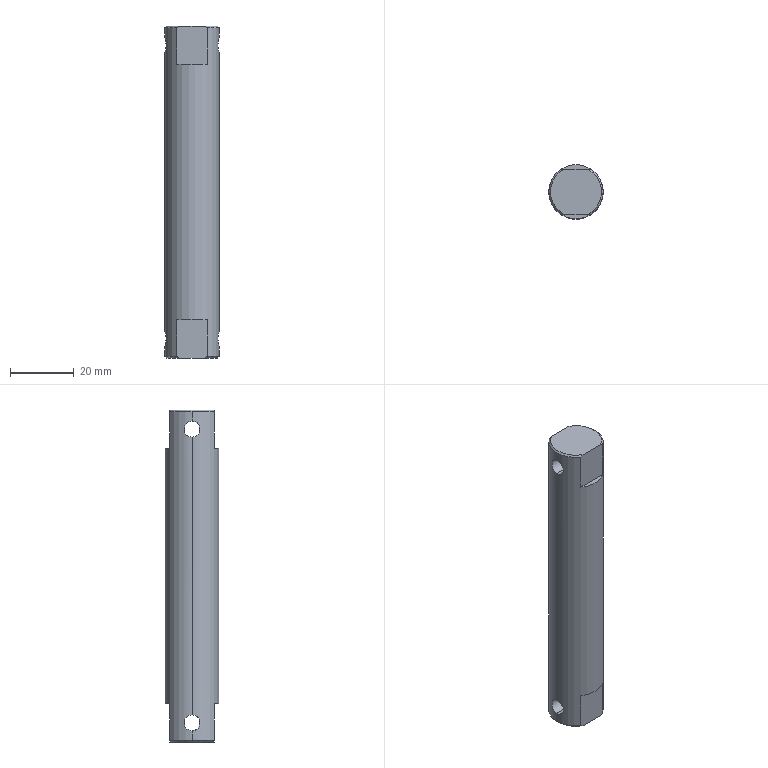Part | SolidWorks | features Chamfer 1, Extrusion 1, HoleWzd 1, ICE 1, MirrorPattern 1 | 1 solid | 22 faces | box 17 x 17 x 104 mm | volume 22466 mm3 | plane 10 | cylinder 6 | cone 6 | commonest cylinder face diameters 5 x4 17 x2
STEP:
#1=CARTESIAN_POINT('',(-8.5,0.,48.5));
#2=VERTEX_POINT('',#1);
#3=CARTESIAN_POINT('',(-8.5,0.,43.5));
#4=VERTEX_POINT('',#3);
#5=CARTESIAN_POINT('',(-8.5,0.,48.5));
#6=CARTESIAN_POINT('',(-8.5,-0.3274,48.5));
#7=CARTESIAN_POINT('',(-8.48,-0.658,48.434));
#8=CARTESIAN_POINT('',(-8.429,-1.11,48.246));
#9=CARTESIAN_POINT('',(-8.408,-1.256,48.168));
#10=CARTESIAN_POINT('',(-8.363,-1.527,47.986));
#11=CARTESIAN_POINT('',(-8.339,-1.652,47.883));
#12=CARTESIAN_POINT('',(-8.29,-1.883,47.653));
#13=CARTESIAN_POINT('',(-8.265,-1.987,47.525));
#14=CARTESIAN_POINT('',(-8.219,-2.168,47.256));
#15=CARTESIAN_POINT('',(-8.198,-2.245,47.113));
#16=CARTESIAN_POINT('',(-8.163,-2.372,46.808));
#17=CARTESIAN_POINT('',(-8.149,-2.419,46.651));
#18=CARTESIAN_POINT('',(-8.129,-2.483,46.331));
#19=CARTESIAN_POINT('',(-8.124,-2.5,46.165));
#20=CARTESIAN_POINT('',(-8.124,-2.5,45.835));
#21=CARTESIAN_POINT('',(-8.129,-2.484,45.673));
#22=CARTESIAN_POINT('',(-8.148,-2.42,45.351));
#23=CARTESIAN_POINT('',(-8.163,-2.371,45.191));
#24=CARTESIAN_POINT('',(-8.216,-2.183,44.739));
#25=CARTESIAN_POINT('',(-8.265,-1.998,44.462));
#26=CARTESIAN_POINT('',(-8.338,-1.654,44.118));
#27=CARTESIAN_POINT('',(-8.363,-1.527,44.013));
#28=CARTESIAN_POINT('',(-8.408,-1.255,43.832));
#29=CARTESIAN_POINT('',(-8.428,-1.112,43.755));
#30=CARTESIAN_POINT('',(-8.463,-0.8109,43.63));
#31=CARTESIAN_POINT('',(-8.477,-0.6512,43.581));
#32=CARTESIAN_POINT('',(-8.495,-0.3296,43.516));
#33=CARTESIAN_POINT('',(-8.5,-0.1661,43.5));
#34=CARTESIAN_POINT('',(-8.5,0.,43.5));
#35=B_SPLINE_CURVE_WITH_KNOTS('',3,(#5,#6,#7,#8,#9,#10,#11,#12,#13,#14,#15,#16,#17,#18,#19,#20,#21,#22,#23,#24,#25,#26,#27,#28,#29,#30,#31,#32,#33,#34),.UNSPECIFIED.,.F.,.F.,(4,2,2,2,2,2,2,2,2,2,2,2,2,2,4),(0.00786,0.008842,0.009333,0.009824,0.01032,0.01081,0.0113,0.01179,0.01228,0.01277,0.01375,0.01424,0.01474,0.01523,0.01572),.UNSPECIFIED.);
#36=EDGE_CURVE('',#2,#4,#35,.T.);
#37=ORIENTED_EDGE('',*,*,#36,.F.);
#38=CARTESIAN_POINT('',(8.5,0.,48.5));
#39=VERTEX_POINT('',#38);
#40=CARTESIAN_POINT('',(8.5,0.,48.5));
#41=DIRECTION('',(1.,0.,0.));
#42=VECTOR('',#41,1000.);
#43=LINE('',#40,#42);
#44=EDGE_CURVE('',#2,#39,#43,.T.);
#45=ORIENTED_EDGE('',*,*,#44,.T.);
#46=CARTESIAN_POINT('',(8.5,0.,43.5));
#47=VERTEX_POINT('',#46);
#48=CARTESIAN_POINT('',(8.5,0.,43.5));
#49=CARTESIAN_POINT('',(8.5,-0.1662,43.5));
#50=CARTESIAN_POINT('',(8.495,-0.3294,43.516));
#51=CARTESIAN_POINT('',(8.477,-0.6502,43.58));
#52=CARTESIAN_POINT('',(8.463,-0.8095,43.629));
#53=CARTESIAN_POINT('',(8.428,-1.112,43.755));
#54=CARTESIAN_POINT('',(8.408,-1.255,43.832));
#55=CARTESIAN_POINT('',(8.363,-1.526,44.013));
#56=CARTESIAN_POINT('',(8.338,-1.654,44.118));
#57=CARTESIAN_POINT('',(8.265,-1.998,44.462));
#58=CARTESIAN_POINT('',(8.216,-2.183,44.74));
#59=CARTESIAN_POINT('',(8.163,-2.371,45.19));
#60=CARTESIAN_POINT('',(8.149,-2.419,45.349));
#61=CARTESIAN_POINT('',(8.129,-2.484,45.672));
#62=CARTESIAN_POINT('',(8.124,-2.5,45.835));
#63=CARTESIAN_POINT('',(8.124,-2.5,46.163));
#64=CARTESIAN_POINT('',(8.129,-2.484,46.33));
#65=CARTESIAN_POINT('',(8.149,-2.419,46.651));
#66=CARTESIAN_POINT('',(8.163,-2.372,46.807));
#67=CARTESIAN_POINT('',(8.216,-2.182,47.263));
#68=CARTESIAN_POINT('',(8.265,-1.998,47.538));
#69=CARTESIAN_POINT('',(8.339,-1.652,47.884));
#70=CARTESIAN_POINT('',(8.363,-1.526,47.987));
#71=CARTESIAN_POINT('',(8.408,-1.256,48.168));
#72=CARTESIAN_POINT('',(8.429,-1.11,48.246));
#73=CARTESIAN_POINT('',(8.463,-0.8084,48.371));
#74=CARTESIAN_POINT('',(8.476,-0.6525,48.419));
#75=CARTESIAN_POINT('',(8.495,-0.3297,48.484));
#76=CARTESIAN_POINT('',(8.5,-0.1637,48.5));
#77=CARTESIAN_POINT('',(8.5,0.,48.5));
#78=B_SPLINE_CURVE_WITH_KNOTS('',3,(#48,#49,#50,#51,#52,#53,#54,#55,#56,#57,#58,#59,#60,#61,#62,#63,#64,#65,#66,#67,#68,#69,#70,#71,#72,#73,#74,#75,#76,#77),.UNSPECIFIED.,.F.,.F.,(4,2,2,2,2,2,2,2,2,2,2,2,2,2,4),(0.,0.0004912,0.0009825,0.001474,0.001965,0.002947,0.003439,0.00393,0.004421,0.004912,0.005895,0.006386,0.006877,0.007369,0.00786),.UNSPECIFIED.);
#79=EDGE_CURVE('',#47,#39,#78,.T.);
#80=ORIENTED_EDGE('',*,*,#79,.F.);
#81=CARTESIAN_POINT('',(8.5,0.,43.5));
#82=DIRECTION('',(1.,0.,0.));
#83=VECTOR('',#82,1000.);
#84=LINE('',#81,#83);
#85=EDGE_CURVE('',#4,#47,#84,.T.);
#86=ORIENTED_EDGE('',*,*,#85,.F.);
#87=EDGE_LOOP('',(#37,#45,#80,#86));
#88=FACE_OUTER_BOUND('',#87,.T.);
#89=CARTESIAN_POINT('',(8.5,0.,46.));
#90=DIRECTION('',(1.,0.,0.));
#91=DIRECTION('',(0.,0.,-1.));
#92=AXIS2_PLACEMENT_3D('',#89,#90,#91);
#93=CYLINDRICAL_SURFACE('',#92,2.5);
#94=ADVANCED_FACE('',(#88),#93,.F.);
#95=CARTESIAN_POINT('',(-8.5,0.,-43.5));
#96=VERTEX_POINT('',#95);
#97=CARTESIAN_POINT('',(-8.5,0.,-48.5));
#98=VERTEX_POINT('',#97);
#99=CARTESIAN_POINT('',(-8.5,0.,-43.5));
#100=CARTESIAN_POINT('',(-8.5,-0.3274,-43.5));
#101=CARTESIAN_POINT('',(-8.48,-0.658,-43.566));
#102=CARTESIAN_POINT('',(-8.429,-1.11,-43.754));
#103=CARTESIAN_POINT('',(-8.408,-1.256,-43.832));
#104=CARTESIAN_POINT('',(-8.363,-1.527,-44.014));
#105=CARTESIAN_POINT('',(-8.339,-1.652,-44.117));
#106=CARTESIAN_POINT('',(-8.29,-1.883,-44.347));
#107=CARTESIAN_POINT('',(-8.265,-1.987,-44.475));
#108=CARTESIAN_POINT('',(-8.219,-2.168,-44.744));
#109=CARTESIAN_POINT('',(-8.198,-2.245,-44.887));
#110=CARTESIAN_POINT('',(-8.163,-2.372,-45.192));
#111=CARTESIAN_POINT('',(-8.149,-2.419,-45.349));
#112=CARTESIAN_POINT('',(-8.129,-2.483,-45.669));
#113=CARTESIAN_POINT('',(-8.124,-2.5,-45.835));
#114=CARTESIAN_POINT('',(-8.124,-2.5,-46.165));
#115=CARTESIAN_POINT('',(-8.129,-2.484,-46.327));
#116=CARTESIAN_POINT('',(-8.148,-2.42,-46.649));
#117=CARTESIAN_POINT('',(-8.163,-2.371,-46.809));
#118=CARTESIAN_POINT('',(-8.216,-2.183,-47.261));
#119=CARTESIAN_POINT('',(-8.265,-1.998,-47.538));
#120=CARTESIAN_POINT('',(-8.338,-1.654,-47.882));
#121=CARTESIAN_POINT('',(-8.363,-1.527,-47.987));
#122=CARTESIAN_POINT('',(-8.408,-1.255,-48.168));
#123=CARTESIAN_POINT('',(-8.428,-1.112,-48.245));
#124=CARTESIAN_POINT('',(-8.463,-0.8109,-48.37));
#125=CARTESIAN_POINT('',(-8.477,-0.6512,-48.419));
#126=CARTESIAN_POINT('',(-8.495,-0.3296,-48.484));
#127=CARTESIAN_POINT('',(-8.5,-0.1661,-48.5));
#128=CARTESIAN_POINT('',(-8.5,0.,-48.5));
#129=B_SPLINE_CURVE_WITH_KNOTS('',3,(#99,#100,#101,#102,#103,#104,#105,#106,#107,#108,#109,#110,#111,#112,#113,#114,#115,#116,#117,#118,#119,#120,#121,#122,#123,#124,#125,#126,#127,#128),.UNSPECIFIED.,.F.,.F.,(4,2,2,2,2,2,2,2,2,2,2,2,2,2,4),(0.00786,0.008842,0.009333,0.009824,0.01032,0.01081,0.0113,0.01179,0.01228,0.01277,0.01375,0.01424,0.01474,0.01523,0.01572),.UNSPECIFIED.);
#130=EDGE_CURVE('',#96,#98,#129,.T.);
#131=ORIENTED_EDGE('',*,*,#130,.F.);
#132=CARTESIAN_POINT('',(8.5,0.,-43.5));
#133=VERTEX_POINT('',#132);
#134=CARTESIAN_POINT('',(8.5,0.,-43.5));
#135=DIRECTION('',(1.,0.,0.));
#136=VECTOR('',#135,1000.);
#137=LINE('',#134,#136);
#138=EDGE_CURVE('',#96,#133,#137,.T.);
#139=ORIENTED_EDGE('',*,*,#138,.T.);
#140=CARTESIAN_POINT('',(8.5,0.,-48.5));
#141=VERTEX_POINT('',#140);
#142=CARTESIAN_POINT('',(8.5,0.,-48.5));
#143=CARTESIAN_POINT('',(8.5,-0.1662,-48.5));
#144=CARTESIAN_POINT('',(8.495,-0.3294,-48.484));
#145=CARTESIAN_POINT('',(8.477,-0.6502,-48.42));
#146=CARTESIAN_POINT('',(8.463,-0.8095,-48.371));
#147=CARTESIAN_POINT('',(8.428,-1.112,-48.245));
#148=CARTESIAN_POINT('',(8.408,-1.255,-48.168));
#149=CARTESIAN_POINT('',(8.363,-1.526,-47.987));
#150=CARTESIAN_POINT('',(8.338,-1.654,-47.882));
#151=CARTESIAN_POINT('',(8.265,-1.998,-47.538));
#152=CARTESIAN_POINT('',(8.216,-2.183,-47.26));
#153=CARTESIAN_POINT('',(8.163,-2.371,-46.81));
#154=CARTESIAN_POINT('',(8.149,-2.419,-46.651));
#155=CARTESIAN_POINT('',(8.129,-2.484,-46.328));
#156=CARTESIAN_POINT('',(8.124,-2.5,-46.165));
#157=CARTESIAN_POINT('',(8.124,-2.5,-45.837));
#158=CARTESIAN_POINT('',(8.129,-2.484,-45.67));
#159=CARTESIAN_POINT('',(8.149,-2.419,-45.349));
#160=CARTESIAN_POINT('',(8.163,-2.372,-45.193));
#161=CARTESIAN_POINT('',(8.216,-2.182,-44.737));
#162=CARTESIAN_POINT('',(8.265,-1.998,-44.462));
#163=CARTESIAN_POINT('',(8.339,-1.652,-44.116));
#164=CARTESIAN_POINT('',(8.363,-1.526,-44.013));
#165=CARTESIAN_POINT('',(8.408,-1.256,-43.832));
#166=CARTESIAN_POINT('',(8.429,-1.11,-43.754));
#167=CARTESIAN_POINT('',(8.463,-0.8084,-43.629));
#168=CARTESIAN_POINT('',(8.476,-0.6525,-43.581));
#169=CARTESIAN_POINT('',(8.495,-0.3297,-43.516));
#170=CARTESIAN_POINT('',(8.5,-0.1637,-43.5));
#171=CARTESIAN_POINT('',(8.5,0.,-43.5));
#172=B_SPLINE_CURVE_WITH_KNOTS('',3,(#142,#143,#144,#145,#146,#147,#148,#149,#150,#151,#152,#153,#154,#155,#156,#157,#158,#159,#160,#161,#162,#163,#164,#165,#166,#167,#168,#169,#170,#171),.UNSPECIFIED.,.F.,.F.,(4,2,2,2,2,2,2,2,2,2,2,2,2,2,4),(0.,0.0004912,0.0009825,0.001474,0.001965,0.002947,0.003439,0.00393,0.004421,0.004912,0.005895,0.006386,0.006877,0.007369,0.00786),.UNSPECIFIED.);
#173=EDGE_CURVE('',#141,#133,#172,.T.);
#174=ORIENTED_EDGE('',*,*,#173,.F.);
#175=CARTESIAN_POINT('',(8.5,0.,-48.5));
#176=DIRECTION('',(1.,0.,0.));
#177=VECTOR('',#176,1000.);
#178=LINE('',#175,#177);
#179=EDGE_CURVE('',#98,#141,#178,.T.);
#180=ORIENTED_EDGE('',*,*,#179,.F.);
#181=EDGE_LOOP('',(#131,#139,#174,#180));
#182=FACE_OUTER_BOUND('',#181,.T.);
#183=CARTESIAN_POINT('',(8.5,0.,-46.));
#184=DIRECTION('',(1.,0.,0.));
#185=DIRECTION('',(0.,0.,-1.));
#186=AXIS2_PLACEMENT_3D('',#183,#184,#185);
#187=CYLINDRICAL_SURFACE('',#186,2.5);
#188=ADVANCED_FACE('',(#182),#187,.F.);
#189=CARTESIAN_POINT('',(-8.,0.,52.));
#190=VERTEX_POINT('',#189);
#191=CARTESIAN_POINT('',(-3.873,-7.,52.));
#192=VERTEX_POINT('',#191);
#193=CARTESIAN_POINT('',(0.,0.,52.));
#194=DIRECTION('',(0.,0.,1.));
#195=DIRECTION('',(1.,0.,0.));
#196=AXIS2_PLACEMENT_3D('',#193,#194,#195);
#197=CIRCLE('',#196,8.);
#198=EDGE_CURVE('',#190,#192,#197,.T.);
#199=ORIENTED_EDGE('',*,*,#198,.F.);
#200=CARTESIAN_POINT('',(-8.5,0.,51.5));
#201=VERTEX_POINT('',#200);
#202=CARTESIAN_POINT('',(-8.,0.,52.));
#203=DIRECTION('',(-0.7071,0.,-0.7071));
#204=VECTOR('',#203,1000.);
#205=LINE('',#202,#204);
#206=EDGE_CURVE('',#190,#201,#205,.T.);
#207=ORIENTED_EDGE('',*,*,#206,.T.);
#208=CARTESIAN_POINT('',(-4.822,-7.,51.5));
#209=VERTEX_POINT('',#208);
#210=CARTESIAN_POINT('',(0.,0.,51.5));
#211=DIRECTION('',(0.,0.,-1.));
#212=DIRECTION('',(1.,0.,0.));
#213=AXIS2_PLACEMENT_3D('',#210,#211,#212);
#214=CIRCLE('',#213,8.5);
#215=EDGE_CURVE('',#209,#201,#214,.T.);
#216=ORIENTED_EDGE('',*,*,#215,.F.);
#217=CARTESIAN_POINT('',(-3.873,-7.,52.));
#218=CARTESIAN_POINT('',(-4.195,-7.,51.844));
#219=CARTESIAN_POINT('',(-4.511,-7.,51.676));
#220=CARTESIAN_POINT('',(-4.822,-7.,51.5));
#221=B_SPLINE_CURVE_WITH_KNOTS('',3,(#217,#218,#219,#220),.UNSPECIFIED.,.F.,.F.,(4,4),(0.,0.001073),.UNSPECIFIED.);
#222=EDGE_CURVE('',#192,#209,#221,.T.);
#223=ORIENTED_EDGE('',*,*,#222,.F.);
#224=EDGE_LOOP('',(#199,#207,#216,#223));
#225=FACE_OUTER_BOUND('',#224,.T.);
#226=CARTESIAN_POINT('',(0.,0.,52.));
#227=DIRECTION('',(0.,0.,-1.));
#228=DIRECTION('',(-1.,0.,0.));
#229=AXIS2_PLACEMENT_3D('',#226,#227,#228);
#230=CONICAL_SURFACE('',#229,8.,0.7854);
#231=ADVANCED_FACE('',(#225),#230,.T.);
#232=CARTESIAN_POINT('',(8.,0.,-52.));
#233=VERTEX_POINT('',#232);
#234=CARTESIAN_POINT('',(3.873,-7.,-52.));
#235=VERTEX_POINT('',#234);
#236=CARTESIAN_POINT('',(0.,0.,-52.));
#237=DIRECTION('',(0.,0.,-1.));
#238=DIRECTION('',(1.,0.,0.));
#239=AXIS2_PLACEMENT_3D('',#236,#237,#238);
#240=CIRCLE('',#239,8.);
#241=EDGE_CURVE('',#233,#235,#240,.T.);
#242=ORIENTED_EDGE('',*,*,#241,.F.);
#243=CARTESIAN_POINT('',(8.5,0.,-51.5));
#244=VERTEX_POINT('',#243);
#245=CARTESIAN_POINT('',(8.5,0.,-51.5));
#246=DIRECTION('',(0.7071,0.,0.7071));
#247=VECTOR('',#246,1000.);
#248=LINE('',#245,#247);
#249=EDGE_CURVE('',#233,#244,#248,.T.);
#250=ORIENTED_EDGE('',*,*,#249,.T.);
#251=CARTESIAN_POINT('',(4.822,-7.,-51.5));
#252=VERTEX_POINT('',#251);
#253=CARTESIAN_POINT('',(0.,0.,-51.5));
#254=DIRECTION('',(0.,0.,1.));
#255=DIRECTION('',(1.,0.,0.));
#256=AXIS2_PLACEMENT_3D('',#253,#254,#255);
#257=CIRCLE('',#256,8.5);
#258=EDGE_CURVE('',#252,#244,#257,.T.);
#259=ORIENTED_EDGE('',*,*,#258,.F.);
#260=CARTESIAN_POINT('',(3.873,-7.,-52.));
#261=CARTESIAN_POINT('',(4.195,-7.,-51.844));
#262=CARTESIAN_POINT('',(4.511,-7.,-51.676));
#263=CARTESIAN_POINT('',(4.822,-7.,-51.5));
#264=B_SPLINE_CURVE_WITH_KNOTS('',3,(#260,#261,#262,#263),.UNSPECIFIED.,.F.,.F.,(4,4),(0.,0.001073),.UNSPECIFIED.);
#265=EDGE_CURVE('',#235,#252,#264,.T.);
#266=ORIENTED_EDGE('',*,*,#265,.F.);
#267=EDGE_LOOP('',(#242,#250,#259,#266));
#268=FACE_OUTER_BOUND('',#267,.T.);
#269=CARTESIAN_POINT('',(0.,0.,-51.5));
#270=DIRECTION('',(0.,0.,1.));
#271=DIRECTION('',(1.,0.,0.));
#272=AXIS2_PLACEMENT_3D('',#269,#270,#271);
#273=CONICAL_SURFACE('',#272,8.5,0.7854);
#274=ADVANCED_FACE('',(#268),#273,.T.);
#275=CARTESIAN_POINT('',(4.822,7.,51.5));
#276=VERTEX_POINT('',#275);
#277=CARTESIAN_POINT('',(8.5,0.,51.5));
#278=VERTEX_POINT('',#277);
#279=CARTESIAN_POINT('',(0.,0.,51.5));
#280=DIRECTION('',(0.,0.,-1.));
#281=DIRECTION('',(1.,0.,0.));
#282=AXIS2_PLACEMENT_3D('',#279,#280,#281);
#283=CIRCLE('',#282,8.5);
#284=EDGE_CURVE('',#276,#278,#283,.T.);
#285=ORIENTED_EDGE('',*,*,#284,.T.);
#286=CARTESIAN_POINT('',(8.5,0.,52.));
#287=DIRECTION('',(0.,0.,-1.));
#288=VECTOR('',#287,1000.);
#289=LINE('',#286,#288);
#290=EDGE_CURVE('',#278,#39,#289,.T.);
#291=ORIENTED_EDGE('',*,*,#290,.T.);
#292=CARTESIAN_POINT('',(8.5,0.,48.5));
#293=CARTESIAN_POINT('',(8.5,0.3274,48.5));
#294=CARTESIAN_POINT('',(8.48,0.658,48.434));
#295=CARTESIAN_POINT('',(8.429,1.11,48.246));
#296=CARTESIAN_POINT('',(8.408,1.256,48.168));
#297=CARTESIAN_POINT('',(8.363,1.527,47.986));
#298=CARTESIAN_POINT('',(8.339,1.652,47.883));
#299=CARTESIAN_POINT('',(8.29,1.883,47.653));
#300=CARTESIAN_POINT('',(8.265,1.987,47.525));
#301=CARTESIAN_POINT('',(8.219,2.168,47.256));
#302=CARTESIAN_POINT('',(8.198,2.245,47.113));
#303=CARTESIAN_POINT('',(8.163,2.372,46.808));
#304=CARTESIAN_POINT('',(8.149,2.419,46.651));
#305=CARTESIAN_POINT('',(8.129,2.483,46.331));
#306=CARTESIAN_POINT('',(8.124,2.5,46.165));
#307=CARTESIAN_POINT('',(8.124,2.5,45.835));
#308=CARTESIAN_POINT('',(8.129,2.484,45.673));
#309=CARTESIAN_POINT('',(8.148,2.42,45.351));
#310=CARTESIAN_POINT('',(8.163,2.371,45.191));
#311=CARTESIAN_POINT('',(8.216,2.183,44.739));
#312=CARTESIAN_POINT('',(8.265,1.998,44.462));
#313=CARTESIAN_POINT('',(8.338,1.654,44.118));
#314=CARTESIAN_POINT('',(8.363,1.527,44.013));
#315=CARTESIAN_POINT('',(8.408,1.255,43.832));
#316=CARTESIAN_POINT('',(8.428,1.112,43.755));
#317=CARTESIAN_POINT('',(8.463,0.8109,43.63));
#318=CARTESIAN_POINT('',(8.477,0.6512,43.581));
#319=CARTESIAN_POINT('',(8.495,0.3296,43.516));
#320=CARTESIAN_POINT('',(8.5,0.1661,43.5));
#321=CARTESIAN_POINT('',(8.5,0.,43.5));
#322=B_SPLINE_CURVE_WITH_KNOTS('',3,(#292,#293,#294,#295,#296,#297,#298,#299,#300,#301,#302,#303,#304,#305,#306,#307,#308,#309,#310,#311,#312,#313,#314,#315,#316,#317,#318,#319,#320,#321),.UNSPECIFIED.,.F.,.F.,(4,2,2,2,2,2,2,2,2,2,2,2,2,2,4),(0.00786,0.008842,0.009333,0.009824,0.01032,0.01081,0.0113,0.01179,0.01228,0.01277,0.01375,0.01424,0.01474,0.01523,0.01572),.UNSPECIFIED.);
#323=EDGE_CURVE('',#39,#47,#322,.T.);
#324=ORIENTED_EDGE('',*,*,#323,.T.);
#325=CARTESIAN_POINT('',(8.5,0.,52.));
#326=DIRECTION('',(0.,0.,-1.));
#327=VECTOR('',#326,1000.);
#328=LINE('',#325,#327);
#329=EDGE_CURVE('',#47,#133,#328,.T.);
#330=ORIENTED_EDGE('',*,*,#329,.T.);
#331=CARTESIAN_POINT('',(8.5,0.,-43.5));
#332=CARTESIAN_POINT('',(8.5,0.3274,-43.5));
#333=CARTESIAN_POINT('',(8.48,0.658,-43.566));
#334=CARTESIAN_POINT('',(8.429,1.11,-43.754));
#335=CARTESIAN_POINT('',(8.408,1.256,-43.832));
#336=CARTESIAN_POINT('',(8.363,1.527,-44.014));
#337=CARTESIAN_POINT('',(8.339,1.652,-44.117));
#338=CARTESIAN_POINT('',(8.29,1.883,-44.347));
#339=CARTESIAN_POINT('',(8.265,1.987,-44.475));
#340=CARTESIAN_POINT('',(8.219,2.168,-44.744));
#341=CARTESIAN_POINT('',(8.198,2.245,-44.887));
#342=CARTESIAN_POINT('',(8.163,2.372,-45.192));
#343=CARTESIAN_POINT('',(8.149,2.419,-45.349));
#344=CARTESIAN_POINT('',(8.129,2.483,-45.669));
#345=CARTESIAN_POINT('',(8.124,2.5,-45.835));
#346=CARTESIAN_POINT('',(8.124,2.5,-46.165));
#347=CARTESIAN_POINT('',(8.129,2.484,-46.327));
#348=CARTESIAN_POINT('',(8.148,2.42,-46.649));
#349=CARTESIAN_POINT('',(8.163,2.371,-46.809));
#350=CARTESIAN_POINT('',(8.216,2.183,-47.261));
#351=CARTESIAN_POINT('',(8.265,1.998,-47.538));
#352=CARTESIAN_POINT('',(8.338,1.654,-47.882));
#353=CARTESIAN_POINT('',(8.363,1.527,-47.987));
#354=CARTESIAN_POINT('',(8.408,1.255,-48.168));
#355=CARTESIAN_POINT('',(8.428,1.112,-48.245));
#356=CARTESIAN_POINT('',(8.463,0.8109,-48.37));
#357=CARTESIAN_POINT('',(8.477,0.6512,-48.419));
#358=CARTESIAN_POINT('',(8.495,0.3296,-48.484));
#359=CARTESIAN_POINT('',(8.5,0.1661,-48.5));
#360=CARTESIAN_POINT('',(8.5,0.,-48.5));
#361=B_SPLINE_CURVE_WITH_KNOTS('',3,(#331,#332,#333,#334,#335,#336,#337,#338,#339,#340,#341,#342,#343,#344,#345,#346,#347,#348,#349,#350,#351,#352,#353,#354,#355,#356,#357,#358,#359,#360),.UNSPECIFIED.,.F.,.F.,(4,2,2,2,2,2,2,2,2,2,2,2,2,2,4),(0.00786,0.008842,0.009333,0.009824,0.01032,0.01081,0.0113,0.01179,0.01228,0.01277,0.01375,0.01424,0.01474,0.01523,0.01572),.UNSPECIFIED.);
#362=EDGE_CURVE('',#133,#141,#361,.T.);
#363=ORIENTED_EDGE('',*,*,#362,.T.);
#364=CARTESIAN_POINT('',(8.5,0.,52.));
#365=DIRECTION('',(0.,0.,-1.));
#366=VECTOR('',#365,1000.);
#367=LINE('',#364,#366);
#368=EDGE_CURVE('',#141,#244,#367,.T.);
#369=ORIENTED_EDGE('',*,*,#368,.T.);
#370=CARTESIAN_POINT('',(4.822,7.,-51.5));
#371=VERTEX_POINT('',#370);
#372=CARTESIAN_POINT('',(0.,0.,-51.5));
#373=DIRECTION('',(0.,0.,1.));
#374=DIRECTION('',(1.,0.,0.));
#375=AXIS2_PLACEMENT_3D('',#372,#373,#374);
#376=CIRCLE('',#375,8.5);
#377=EDGE_CURVE('',#244,#371,#376,.T.);
#378=ORIENTED_EDGE('',*,*,#377,.T.);
#379=CARTESIAN_POINT('',(4.822,7.,-40.));
#380=VERTEX_POINT('',#379);
#381=CARTESIAN_POINT('',(4.822,7.,52.));
#382=DIRECTION('',(0.,0.,-1.));
#383=VECTOR('',#382,1000.);
#384=LINE('',#381,#383);
#385=EDGE_CURVE('',#380,#371,#384,.T.);
#386=ORIENTED_EDGE('',*,*,#385,.F.);
#387=CARTESIAN_POINT('',(-4.822,7.,-40.));
#388=VERTEX_POINT('',#387);
#389=CARTESIAN_POINT('',(0.,0.,-40.));
#390=DIRECTION('',(0.,0.,-1.));
#391=DIRECTION('',(-1.,0.,0.));
#392=AXIS2_PLACEMENT_3D('',#389,#390,#391);
#393=CIRCLE('',#392,8.5);
#394=EDGE_CURVE('',#388,#380,#393,.T.);
#395=ORIENTED_EDGE('',*,*,#394,.F.);
#396=CARTESIAN_POINT('',(-4.822,7.,-51.5));
#397=VERTEX_POINT('',#396);
#398=CARTESIAN_POINT('',(-4.822,7.,52.));
#399=DIRECTION('',(0.,0.,1.));
#400=VECTOR('',#399,1000.);
#401=LINE('',#398,#400);
#402=EDGE_CURVE('',#397,#388,#401,.T.);
#403=ORIENTED_EDGE('',*,*,#402,.F.);
#404=CARTESIAN_POINT('',(-8.5,0.,-51.5));
#405=VERTEX_POINT('',#404);
#406=CARTESIAN_POINT('',(0.,0.,-51.5));
#407=DIRECTION('',(0.,0.,1.));
#408=DIRECTION('',(1.,0.,0.));
#409=AXIS2_PLACEMENT_3D('',#406,#407,#408);
#410=CIRCLE('',#409,8.5);
#411=EDGE_CURVE('',#397,#405,#410,.T.);
#412=ORIENTED_EDGE('',*,*,#411,.T.);
#413=CARTESIAN_POINT('',(-8.5,0.,52.));
#414=DIRECTION('',(0.,0.,-1.));
#415=VECTOR('',#414,1000.);
#416=LINE('',#413,#415);
#417=EDGE_CURVE('',#98,#405,#416,.T.);
#418=ORIENTED_EDGE('',*,*,#417,.F.);
#419=CARTESIAN_POINT('',(-8.5,0.,-48.5));
#420=CARTESIAN_POINT('',(-8.5,0.1662,-48.5));
#421=CARTESIAN_POINT('',(-8.495,0.3294,-48.484));
#422=CARTESIAN_POINT('',(-8.477,0.6502,-48.42));
#423=CARTESIAN_POINT('',(-8.463,0.8095,-48.371));
#424=CARTESIAN_POINT('',(-8.428,1.112,-48.245));
#425=CARTESIAN_POINT('',(-8.408,1.255,-48.168));
#426=CARTESIAN_POINT('',(-8.363,1.526,-47.987));
#427=CARTESIAN_POINT('',(-8.338,1.654,-47.882));
#428=CARTESIAN_POINT('',(-8.265,1.998,-47.538));
#429=CARTESIAN_POINT('',(-8.216,2.183,-47.26));
#430=CARTESIAN_POINT('',(-8.163,2.371,-46.81));
#431=CARTESIAN_POINT('',(-8.149,2.419,-46.651));
#432=CARTESIAN_POINT('',(-8.129,2.484,-46.328));
#433=CARTESIAN_POINT('',(-8.124,2.5,-46.165));
#434=CARTESIAN_POINT('',(-8.124,2.5,-45.837));
#435=CARTESIAN_POINT('',(-8.129,2.484,-45.67));
#436=CARTESIAN_POINT('',(-8.149,2.419,-45.349));
#437=CARTESIAN_POINT('',(-8.163,2.372,-45.193));
#438=CARTESIAN_POINT('',(-8.216,2.182,-44.737));
#439=CARTESIAN_POINT('',(-8.265,1.998,-44.462));
#440=CARTESIAN_POINT('',(-8.339,1.652,-44.116));
#441=CARTESIAN_POINT('',(-8.363,1.526,-44.013));
#442=CARTESIAN_POINT('',(-8.408,1.256,-43.832));
#443=CARTESIAN_POINT('',(-8.429,1.11,-43.754));
#444=CARTESIAN_POINT('',(-8.463,0.8084,-43.629));
#445=CARTESIAN_POINT('',(-8.476,0.6525,-43.581));
#446=CARTESIAN_POINT('',(-8.495,0.3297,-43.516));
#447=CARTESIAN_POINT('',(-8.5,0.1637,-43.5));
#448=CARTESIAN_POINT('',(-8.5,0.,-43.5));
#449=B_SPLINE_CURVE_WITH_KNOTS('',3,(#419,#420,#421,#422,#423,#424,#425,#426,#427,#428,#429,#430,#431,#432,#433,#434,#435,#436,#437,#438,#439,#440,#441,#442,#443,#444,#445,#446,#447,#448),.UNSPECIFIED.,.F.,.F.,(4,2,2,2,2,2,2,2,2,2,2,2,2,2,4),(0.,0.0004912,0.0009825,0.001474,0.001965,0.002947,0.003439,0.00393,0.004421,0.004912,0.005895,0.006386,0.006877,0.007369,0.00786),.UNSPECIFIED.);
#450=EDGE_CURVE('',#98,#96,#449,.T.);
#451=ORIENTED_EDGE('',*,*,#450,.T.);
#452=CARTESIAN_POINT('',(-8.5,0.,52.));
#453=DIRECTION('',(0.,0.,-1.));
#454=VECTOR('',#453,1000.);
#455=LINE('',#452,#454);
#456=EDGE_CURVE('',#4,#96,#455,.T.);
#457=ORIENTED_EDGE('',*,*,#456,.F.);
#458=CARTESIAN_POINT('',(-8.5,0.,43.5));
#459=CARTESIAN_POINT('',(-8.5,0.1662,43.5));
#460=CARTESIAN_POINT('',(-8.495,0.3294,43.516));
#461=CARTESIAN_POINT('',(-8.477,0.6502,43.58));
#462=CARTESIAN_POINT('',(-8.463,0.8095,43.629));
#463=CARTESIAN_POINT('',(-8.428,1.112,43.755));
#464=CARTESIAN_POINT('',(-8.408,1.255,43.832));
#465=CARTESIAN_POINT('',(-8.363,1.526,44.013));
#466=CARTESIAN_POINT('',(-8.338,1.654,44.118));
#467=CARTESIAN_POINT('',(-8.265,1.998,44.462));
#468=CARTESIAN_POINT('',(-8.216,2.183,44.74));
#469=CARTESIAN_POINT('',(-8.163,2.371,45.19));
#470=CARTESIAN_POINT('',(-8.149,2.419,45.349));
#471=CARTESIAN_POINT('',(-8.129,2.484,45.672));
#472=CARTESIAN_POINT('',(-8.124,2.5,45.835));
#473=CARTESIAN_POINT('',(-8.124,2.5,46.163));
#474=CARTESIAN_POINT('',(-8.129,2.484,46.33));
#475=CARTESIAN_POINT('',(-8.149,2.419,46.651));
#476=CARTESIAN_POINT('',(-8.163,2.372,46.807));
#477=CARTESIAN_POINT('',(-8.216,2.182,47.263));
#478=CARTESIAN_POINT('',(-8.265,1.998,47.538));
#479=CARTESIAN_POINT('',(-8.339,1.652,47.884));
#480=CARTESIAN_POINT('',(-8.363,1.526,47.987));
#481=CARTESIAN_POINT('',(-8.408,1.256,48.168));
#482=CARTESIAN_POINT('',(-8.429,1.11,48.246));
#483=CARTESIAN_POINT('',(-8.463,0.8084,48.371));
#484=CARTESIAN_POINT('',(-8.476,0.6525,48.419));
#485=CARTESIAN_POINT('',(-8.495,0.3297,48.484));
#486=CARTESIAN_POINT('',(-8.5,0.1637,48.5));
#487=CARTESIAN_POINT('',(-8.5,0.,48.5));
#488=B_SPLINE_CURVE_WITH_KNOTS('',3,(#458,#459,#460,#461,#462,#463,#464,#465,#466,#467,#468,#469,#470,#471,#472,#473,#474,#475,#476,#477,#478,#479,#480,#481,#482,#483,#484,#485,#486,#487),.UNSPECIFIED.,.F.,.F.,(4,2,2,2,2,2,2,2,2,2,2,2,2,2,4),(0.,0.0004912,0.0009825,0.001474,0.001965,0.002947,0.003439,0.00393,0.004421,0.004912,0.005895,0.006386,0.006877,0.007369,0.00786),.UNSPECIFIED.);
#489=EDGE_CURVE('',#4,#2,#488,.T.);
#490=ORIENTED_EDGE('',*,*,#489,.T.);
#491=CARTESIAN_POINT('',(-8.5,0.,52.));
#492=DIRECTION('',(0.,0.,-1.));
#493=VECTOR('',#492,1000.);
#494=LINE('',#491,#493);
#495=EDGE_CURVE('',#201,#2,#494,.T.);
#496=ORIENTED_EDGE('',*,*,#495,.F.);
#497=CARTESIAN_POINT('',(-4.822,7.,51.5));
#498=VERTEX_POINT('',#497);
#499=CARTESIAN_POINT('',(0.,0.,51.5));
#500=DIRECTION('',(0.,0.,-1.));
#501=DIRECTION('',(1.,0.,0.));
#502=AXIS2_PLACEMENT_3D('',#499,#500,#501);
#503=CIRCLE('',#502,8.5);
#504=EDGE_CURVE('',#201,#498,#503,.T.);
#505=ORIENTED_EDGE('',*,*,#504,.T.);
#506=CARTESIAN_POINT('',(-4.822,7.,40.));
#507=VERTEX_POINT('',#506);
#508=CARTESIAN_POINT('',(-4.822,7.,52.));
#509=DIRECTION('',(0.,0.,-1.));
#510=VECTOR('',#509,1000.);
#511=LINE('',#508,#510);
#512=EDGE_CURVE('',#498,#507,#511,.T.);
#513=ORIENTED_EDGE('',*,*,#512,.T.);
#514=CARTESIAN_POINT('',(4.822,7.,40.));
#515=VERTEX_POINT('',#514);
#516=CARTESIAN_POINT('',(0.,0.,40.));
#517=DIRECTION('',(0.,0.,1.));
#518=DIRECTION('',(1.,0.,0.));
#519=AXIS2_PLACEMENT_3D('',#516,#517,#518);
#520=CIRCLE('',#519,8.5);
#521=EDGE_CURVE('',#515,#507,#520,.T.);
#522=ORIENTED_EDGE('',*,*,#521,.F.);
#523=CARTESIAN_POINT('',(4.822,7.,52.));
#524=DIRECTION('',(0.,0.,1.));
#525=VECTOR('',#524,1000.);
#526=LINE('',#523,#525);
#527=EDGE_CURVE('',#515,#276,#526,.T.);
#528=ORIENTED_EDGE('',*,*,#527,.T.);
#529=EDGE_LOOP('',(#285,#291,#324,#330,#363,#369,#378,#386,#395,#403,#412,#418,#451,#457,#490,#496,#505,#513,#522,#528));
#530=FACE_OUTER_BOUND('',#529,.T.);
#531=CARTESIAN_POINT('',(0.,0.,52.));
#532=DIRECTION('',(0.,0.,-1.));
#533=DIRECTION('',(-1.,0.,0.));
#534=AXIS2_PLACEMENT_3D('',#531,#532,#533);
#535=CYLINDRICAL_SURFACE('',#534,8.5);
#536=ADVANCED_FACE('',(#530),#535,.T.);
#537=ORIENTED_EDGE('',*,*,#290,.F.);
#538=CARTESIAN_POINT('',(4.822,-7.,51.5));
#539=VERTEX_POINT('',#538);
#540=CARTESIAN_POINT('',(0.,0.,51.5));
#541=DIRECTION('',(0.,0.,-1.));
#542=DIRECTION('',(1.,0.,0.));
#543=AXIS2_PLACEMENT_3D('',#540,#541,#542);
#544=CIRCLE('',#543,8.5);
#545=EDGE_CURVE('',#278,#539,#544,.T.);
#546=ORIENTED_EDGE('',*,*,#545,.T.);
#547=CARTESIAN_POINT('',(4.822,-7.,40.));
#548=VERTEX_POINT('',#547);
#549=CARTESIAN_POINT('',(4.822,-7.,52.));
#550=DIRECTION('',(0.,0.,-1.));
#551=VECTOR('',#550,1000.);
#552=LINE('',#549,#551);
#553=EDGE_CURVE('',#539,#548,#552,.T.);
#554=ORIENTED_EDGE('',*,*,#553,.T.);
#555=CARTESIAN_POINT('',(-4.822,-7.,40.));
#556=VERTEX_POINT('',#555);
#557=CARTESIAN_POINT('',(0.,0.,40.));
#558=DIRECTION('',(0.,0.,-1.));
#559=DIRECTION('',(-1.,0.,0.));
#560=AXIS2_PLACEMENT_3D('',#557,#558,#559);
#561=CIRCLE('',#560,8.5);
#562=EDGE_CURVE('',#548,#556,#561,.T.);
#563=ORIENTED_EDGE('',*,*,#562,.T.);
#564=CARTESIAN_POINT('',(-4.822,-7.,52.));
#565=DIRECTION('',(0.,0.,1.));
#566=VECTOR('',#565,1000.);
#567=LINE('',#564,#566);
#568=EDGE_CURVE('',#556,#209,#567,.T.);
#569=ORIENTED_EDGE('',*,*,#568,.T.);
#570=ORIENTED_EDGE('',*,*,#215,.T.);
#571=ORIENTED_EDGE('',*,*,#495,.T.);
#572=ORIENTED_EDGE('',*,*,#36,.T.);
#573=ORIENTED_EDGE('',*,*,#456,.T.);
#574=ORIENTED_EDGE('',*,*,#130,.T.);
#575=ORIENTED_EDGE('',*,*,#417,.T.);
#576=CARTESIAN_POINT('',(-4.822,-7.,-51.5));
#577=VERTEX_POINT('',#576);
#578=CARTESIAN_POINT('',(0.,0.,-51.5));
#579=DIRECTION('',(0.,0.,1.));
#580=DIRECTION('',(1.,0.,0.));
#581=AXIS2_PLACEMENT_3D('',#578,#579,#580);
#582=CIRCLE('',#581,8.5);
#583=EDGE_CURVE('',#405,#577,#582,.T.);
#584=ORIENTED_EDGE('',*,*,#583,.T.);
#585=CARTESIAN_POINT('',(-4.822,-7.,-40.));
#586=VERTEX_POINT('',#585);
#587=CARTESIAN_POINT('',(-4.822,-7.,52.));
#588=DIRECTION('',(0.,0.,-1.));
#589=VECTOR('',#588,1000.);
#590=LINE('',#587,#589);
#591=EDGE_CURVE('',#586,#577,#590,.T.);
#592=ORIENTED_EDGE('',*,*,#591,.F.);
#593=CARTESIAN_POINT('',(4.822,-7.,-40.));
#594=VERTEX_POINT('',#593);
#595=CARTESIAN_POINT('',(0.,0.,-40.));
#596=DIRECTION('',(0.,0.,1.));
#597=DIRECTION('',(1.,0.,0.));
#598=AXIS2_PLACEMENT_3D('',#595,#596,#597);
#599=CIRCLE('',#598,8.5);
#600=EDGE_CURVE('',#586,#594,#599,.T.);
#601=ORIENTED_EDGE('',*,*,#600,.T.);
#602=CARTESIAN_POINT('',(4.822,-7.,52.));
#603=DIRECTION('',(0.,0.,1.));
#604=VECTOR('',#603,1000.);
#605=LINE('',#602,#604);
#606=EDGE_CURVE('',#252,#594,#605,.T.);
#607=ORIENTED_EDGE('',*,*,#606,.F.);
#608=ORIENTED_EDGE('',*,*,#258,.T.);
#609=ORIENTED_EDGE('',*,*,#368,.F.);
#610=ORIENTED_EDGE('',*,*,#173,.T.);
#611=ORIENTED_EDGE('',*,*,#329,.F.);
#612=ORIENTED_EDGE('',*,*,#79,.T.);
#613=EDGE_LOOP('',(#537,#546,#554,#563,#569,#570,#571,#572,#573,#574,#575,#584,#592,#601,#607,#608,#609,#610,#611,#612));
#614=FACE_OUTER_BOUND('',#613,.T.);
#615=CARTESIAN_POINT('',(0.,0.,52.));
#616=DIRECTION('',(0.,0.,-1.));
#617=DIRECTION('',(-1.,0.,0.));
#618=AXIS2_PLACEMENT_3D('',#615,#616,#617);
#619=CYLINDRICAL_SURFACE('',#618,8.5);
#620=ADVANCED_FACE('',(#614),#619,.T.);
#621=CARTESIAN_POINT('',(-3.873,-7.,-52.));
#622=VERTEX_POINT('',#621);
#623=CARTESIAN_POINT('',(0.,-7.,-52.));
#624=DIRECTION('',(1.,0.,0.));
#625=VECTOR('',#624,1000.);
#626=LINE('',#623,#625);
#627=EDGE_CURVE('',#622,#235,#626,.T.);
#628=ORIENTED_EDGE('',*,*,#627,.F.);
#629=CARTESIAN_POINT('',(-3.873,7.,-52.));
#630=VERTEX_POINT('',#629);
#631=CARTESIAN_POINT('',(0.,0.,-52.));
#632=DIRECTION('',(0.,0.,-1.));
#633=DIRECTION('',(1.,0.,0.));
#634=AXIS2_PLACEMENT_3D('',#631,#632,#633);
#635=CIRCLE('',#634,8.);
#636=EDGE_CURVE('',#622,#630,#635,.T.);
#637=ORIENTED_EDGE('',*,*,#636,.T.);
#638=CARTESIAN_POINT('',(3.873,7.,-52.));
#639=VERTEX_POINT('',#638);
#640=CARTESIAN_POINT('',(0.,7.,-52.));
#641=DIRECTION('',(-1.,0.,0.));
#642=VECTOR('',#641,1000.);
#643=LINE('',#640,#642);
#644=EDGE_CURVE('',#639,#630,#643,.T.);
#645=ORIENTED_EDGE('',*,*,#644,.F.);
#646=CARTESIAN_POINT('',(0.,0.,-52.));
#647=DIRECTION('',(0.,0.,-1.));
#648=DIRECTION('',(1.,0.,0.));
#649=AXIS2_PLACEMENT_3D('',#646,#647,#648);
#650=CIRCLE('',#649,8.);
#651=EDGE_CURVE('',#639,#233,#650,.T.);
#652=ORIENTED_EDGE('',*,*,#651,.T.);
#653=ORIENTED_EDGE('',*,*,#241,.T.);
#654=EDGE_LOOP('',(#628,#637,#645,#652,#653));
#655=FACE_OUTER_BOUND('',#654,.T.);
#656=CARTESIAN_POINT('',(0.,0.,-52.));
#657=DIRECTION('',(0.,0.,1.));
#658=DIRECTION('',(1.,0.,0.));
#659=AXIS2_PLACEMENT_3D('',#656,#657,#658);
#660=PLANE('',#659);
#661=ADVANCED_FACE('',(#655),#660,.F.);
#662=CARTESIAN_POINT('',(3.873,-7.,52.));
#663=VERTEX_POINT('',#662);
#664=CARTESIAN_POINT('',(0.,-7.,52.));
#665=DIRECTION('',(-1.,0.,0.));
#666=VECTOR('',#665,1000.);
#667=LINE('',#664,#666);
#668=EDGE_CURVE('',#663,#192,#667,.T.);
#669=ORIENTED_EDGE('',*,*,#668,.F.);
#670=CARTESIAN_POINT('',(3.873,7.,52.));
#671=VERTEX_POINT('',#670);
#672=CARTESIAN_POINT('',(0.,0.,52.));
#673=DIRECTION('',(0.,0.,1.));
#674=DIRECTION('',(1.,0.,0.));
#675=AXIS2_PLACEMENT_3D('',#672,#673,#674);
#676=CIRCLE('',#675,8.);
#677=EDGE_CURVE('',#663,#671,#676,.T.);
#678=ORIENTED_EDGE('',*,*,#677,.T.);
#679=CARTESIAN_POINT('',(-3.873,7.,52.));
#680=VERTEX_POINT('',#679);
#681=CARTESIAN_POINT('',(0.,7.,52.));
#682=DIRECTION('',(1.,0.,0.));
#683=VECTOR('',#682,1000.);
#684=LINE('',#681,#683);
#685=EDGE_CURVE('',#680,#671,#684,.T.);
#686=ORIENTED_EDGE('',*,*,#685,.F.);
#687=CARTESIAN_POINT('',(0.,0.,52.));
#688=DIRECTION('',(0.,0.,1.));
#689=DIRECTION('',(1.,0.,0.));
#690=AXIS2_PLACEMENT_3D('',#687,#688,#689);
#691=CIRCLE('',#690,8.);
#692=EDGE_CURVE('',#680,#190,#691,.T.);
#693=ORIENTED_EDGE('',*,*,#692,.T.);
#694=ORIENTED_EDGE('',*,*,#198,.T.);
#695=EDGE_LOOP('',(#669,#678,#686,#693,#694));
#696=FACE_OUTER_BOUND('',#695,.T.);
#697=CARTESIAN_POINT('',(0.,0.,52.));
#698=DIRECTION('',(0.,0.,1.));
#699=DIRECTION('',(1.,0.,0.));
#700=AXIS2_PLACEMENT_3D('',#697,#698,#699);
#701=PLANE('',#700);
#702=ADVANCED_FACE('',(#696),#701,.T.);
#703=ORIENTED_EDGE('',*,*,#521,.T.);
#704=CARTESIAN_POINT('',(-12.5,7.,40.));
#705=DIRECTION('',(1.,0.,0.));
#706=VECTOR('',#705,1000.);
#707=LINE('',#704,#706);
#708=EDGE_CURVE('',#507,#515,#707,.T.);
#709=ORIENTED_EDGE('',*,*,#708,.T.);
#710=EDGE_LOOP('',(#703,#709));
#711=FACE_OUTER_BOUND('',#710,.T.);
#712=CARTESIAN_POINT('',(0.,0.,40.));
#713=DIRECTION('',(0.,0.,1.));
#714=DIRECTION('',(1.,0.,0.));
#715=AXIS2_PLACEMENT_3D('',#712,#713,#714);
#716=PLANE('',#715);
#717=ADVANCED_FACE('',(#711),#716,.T.);
#718=ORIENTED_EDGE('',*,*,#685,.T.);
#719=CARTESIAN_POINT('',(3.873,7.,52.));
#720=CARTESIAN_POINT('',(4.195,7.,51.844));
#721=CARTESIAN_POINT('',(4.511,7.,51.676));
#722=CARTESIAN_POINT('',(4.822,7.,51.5));
#723=B_SPLINE_CURVE_WITH_KNOTS('',3,(#719,#720,#721,#722),.UNSPECIFIED.,.F.,.F.,(4,4),(0.,0.001073),.UNSPECIFIED.);
#724=EDGE_CURVE('',#671,#276,#723,.T.);
#725=ORIENTED_EDGE('',*,*,#724,.T.);
#726=ORIENTED_EDGE('',*,*,#527,.F.);
#727=ORIENTED_EDGE('',*,*,#708,.F.);
#728=ORIENTED_EDGE('',*,*,#512,.F.);
#729=CARTESIAN_POINT('',(-4.822,7.,51.5));
#730=CARTESIAN_POINT('',(-4.511,7.,51.676));
#731=CARTESIAN_POINT('',(-4.195,7.,51.844));
#732=CARTESIAN_POINT('',(-3.873,7.,52.));
#733=B_SPLINE_CURVE_WITH_KNOTS('',3,(#729,#730,#731,#732),.UNSPECIFIED.,.F.,.F.,(4,4),(0.,0.001073),.UNSPECIFIED.);
#734=EDGE_CURVE('',#498,#680,#733,.T.);
#735=ORIENTED_EDGE('',*,*,#734,.T.);
#736=EDGE_LOOP('',(#718,#725,#726,#727,#728,#735));
#737=FACE_OUTER_BOUND('',#736,.T.);
#738=CARTESIAN_POINT('',(-12.5,7.,40.));
#739=DIRECTION('',(0.,-1.,0.));
#740=DIRECTION('',(0.,0.,-1.));
#741=AXIS2_PLACEMENT_3D('',#738,#739,#740);
#742=PLANE('',#741);
#743=ADVANCED_FACE('',(#737),#742,.F.);
#744=CARTESIAN_POINT('',(-12.5,-7.,40.));
#745=DIRECTION('',(-1.,0.,0.));
#746=VECTOR('',#745,1000.);
#747=LINE('',#744,#746);
#748=EDGE_CURVE('',#548,#556,#747,.T.);
#749=ORIENTED_EDGE('',*,*,#748,.T.);
#750=ORIENTED_EDGE('',*,*,#562,.F.);
#751=EDGE_LOOP('',(#749,#750));
#752=FACE_OUTER_BOUND('',#751,.T.);
#753=CARTESIAN_POINT('',(0.,0.,40.));
#754=DIRECTION('',(0.,0.,-1.));
#755=DIRECTION('',(-1.,0.,0.));
#756=AXIS2_PLACEMENT_3D('',#753,#754,#755);
#757=PLANE('',#756);
#758=ADVANCED_FACE('',(#752),#757,.F.);
#759=ORIENTED_EDGE('',*,*,#553,.F.);
#760=CARTESIAN_POINT('',(4.822,-7.,51.5));
#761=CARTESIAN_POINT('',(4.511,-7.,51.676));
#762=CARTESIAN_POINT('',(4.195,-7.,51.844));
#763=CARTESIAN_POINT('',(3.873,-7.,52.));
#764=B_SPLINE_CURVE_WITH_KNOTS('',3,(#760,#761,#762,#763),.UNSPECIFIED.,.F.,.F.,(4,4),(0.,0.001073),.UNSPECIFIED.);
#765=EDGE_CURVE('',#539,#663,#764,.T.);
#766=ORIENTED_EDGE('',*,*,#765,.T.);
#767=ORIENTED_EDGE('',*,*,#668,.T.);
#768=ORIENTED_EDGE('',*,*,#222,.T.);
#769=ORIENTED_EDGE('',*,*,#568,.F.);
#770=ORIENTED_EDGE('',*,*,#748,.F.);
#771=EDGE_LOOP('',(#759,#766,#767,#768,#769,#770));
#772=FACE_OUTER_BOUND('',#771,.T.);
#773=CARTESIAN_POINT('',(-12.5,-7.,40.));
#774=DIRECTION('',(0.,1.,0.));
#775=DIRECTION('',(0.,0.,1.));
#776=AXIS2_PLACEMENT_3D('',#773,#774,#775);
#777=PLANE('',#776);
#778=ADVANCED_FACE('',(#772),#777,.F.);
#779=ORIENTED_EDGE('',*,*,#394,.T.);
#780=CARTESIAN_POINT('',(-12.5,7.,-40.));
#781=DIRECTION('',(1.,0.,0.));
#782=VECTOR('',#781,1000.);
#783=LINE('',#780,#782);
#784=EDGE_CURVE('',#388,#380,#783,.T.);
#785=ORIENTED_EDGE('',*,*,#784,.F.);
#786=EDGE_LOOP('',(#779,#785));
#787=FACE_OUTER_BOUND('',#786,.T.);
#788=CARTESIAN_POINT('',(0.,0.,-40.));
#789=DIRECTION('',(0.,0.,-1.));
#790=DIRECTION('',(1.,0.,0.));
#791=AXIS2_PLACEMENT_3D('',#788,#789,#790);
#792=PLANE('',#791);
#793=ADVANCED_FACE('',(#787),#792,.T.);
#794=ORIENTED_EDGE('',*,*,#644,.T.);
#795=CARTESIAN_POINT('',(-3.873,7.,-52.));
#796=CARTESIAN_POINT('',(-4.195,7.,-51.844));
#797=CARTESIAN_POINT('',(-4.511,7.,-51.676));
#798=CARTESIAN_POINT('',(-4.822,7.,-51.5));
#799=B_SPLINE_CURVE_WITH_KNOTS('',3,(#795,#796,#797,#798),.UNSPECIFIED.,.F.,.F.,(4,4),(0.,0.001073),.UNSPECIFIED.);
#800=EDGE_CURVE('',#630,#397,#799,.T.);
#801=ORIENTED_EDGE('',*,*,#800,.T.);
#802=ORIENTED_EDGE('',*,*,#402,.T.);
#803=ORIENTED_EDGE('',*,*,#784,.T.);
#804=ORIENTED_EDGE('',*,*,#385,.T.);
#805=CARTESIAN_POINT('',(4.822,7.,-51.5));
#806=CARTESIAN_POINT('',(4.511,7.,-51.676));
#807=CARTESIAN_POINT('',(4.195,7.,-51.844));
#808=CARTESIAN_POINT('',(3.873,7.,-52.));
#809=B_SPLINE_CURVE_WITH_KNOTS('',3,(#805,#806,#807,#808),.UNSPECIFIED.,.F.,.F.,(4,4),(0.,0.001073),.UNSPECIFIED.);
#810=EDGE_CURVE('',#371,#639,#809,.T.);
#811=ORIENTED_EDGE('',*,*,#810,.T.);
#812=EDGE_LOOP('',(#794,#801,#802,#803,#804,#811));
#813=FACE_OUTER_BOUND('',#812,.T.);
#814=CARTESIAN_POINT('',(-12.5,7.,-40.));
#815=DIRECTION('',(0.,1.,0.));
#816=DIRECTION('',(0.,0.,1.));
#817=AXIS2_PLACEMENT_3D('',#814,#815,#816);
#818=PLANE('',#817);
#819=ADVANCED_FACE('',(#813),#818,.T.);
#820=CARTESIAN_POINT('',(-12.5,-7.,-40.));
#821=DIRECTION('',(-1.,0.,0.));
#822=VECTOR('',#821,1000.);
#823=LINE('',#820,#822);
#824=EDGE_CURVE('',#594,#586,#823,.T.);
#825=ORIENTED_EDGE('',*,*,#824,.F.);
#826=ORIENTED_EDGE('',*,*,#600,.F.);
#827=EDGE_LOOP('',(#825,#826));
#828=FACE_OUTER_BOUND('',#827,.T.);
#829=CARTESIAN_POINT('',(0.,0.,-40.));
#830=DIRECTION('',(0.,0.,1.));
#831=DIRECTION('',(-1.,0.,0.));
#832=AXIS2_PLACEMENT_3D('',#829,#830,#831);
#833=PLANE('',#832);
#834=ADVANCED_FACE('',(#828),#833,.F.);
#835=ORIENTED_EDGE('',*,*,#591,.T.);
#836=CARTESIAN_POINT('',(-4.822,-7.,-51.5));
#837=CARTESIAN_POINT('',(-4.511,-7.,-51.676));
#838=CARTESIAN_POINT('',(-4.195,-7.,-51.844));
#839=CARTESIAN_POINT('',(-3.873,-7.,-52.));
#840=B_SPLINE_CURVE_WITH_KNOTS('',3,(#836,#837,#838,#839),.UNSPECIFIED.,.F.,.F.,(4,4),(0.,0.001073),.UNSPECIFIED.);
#841=EDGE_CURVE('',#577,#622,#840,.T.);
#842=ORIENTED_EDGE('',*,*,#841,.T.);
#843=ORIENTED_EDGE('',*,*,#627,.T.);
#844=ORIENTED_EDGE('',*,*,#265,.T.);
#845=ORIENTED_EDGE('',*,*,#606,.T.);
#846=ORIENTED_EDGE('',*,*,#824,.T.);
#847=EDGE_LOOP('',(#835,#842,#843,#844,#845,#846));
#848=FACE_OUTER_BOUND('',#847,.T.);
#849=CARTESIAN_POINT('',(-12.5,-7.,-40.));
#850=DIRECTION('',(0.,-1.,0.));
#851=DIRECTION('',(0.,0.,-1.));
#852=AXIS2_PLACEMENT_3D('',#849,#850,#851);
#853=PLANE('',#852);
#854=ADVANCED_FACE('',(#848),#853,.T.);
#855=ORIENTED_EDGE('',*,*,#800,.F.);
#856=ORIENTED_EDGE('',*,*,#636,.F.);
#857=ORIENTED_EDGE('',*,*,#841,.F.);
#858=ORIENTED_EDGE('',*,*,#583,.F.);
#859=ORIENTED_EDGE('',*,*,#411,.F.);
#860=EDGE_LOOP('',(#855,#856,#857,#858,#859));
#861=FACE_OUTER_BOUND('',#860,.T.);
#862=CARTESIAN_POINT('',(0.,0.,-51.5));
#863=DIRECTION('',(0.,0.,1.));
#864=DIRECTION('',(1.,0.,0.));
#865=AXIS2_PLACEMENT_3D('',#862,#863,#864);
#866=CONICAL_SURFACE('',#865,8.5,0.7854);
#867=ADVANCED_FACE('',(#861),#866,.T.);
#868=ORIENTED_EDGE('',*,*,#249,.F.);
#869=ORIENTED_EDGE('',*,*,#651,.F.);
#870=ORIENTED_EDGE('',*,*,#810,.F.);
#871=ORIENTED_EDGE('',*,*,#377,.F.);
#872=EDGE_LOOP('',(#868,#869,#870,#871));
#873=FACE_OUTER_BOUND('',#872,.T.);
#874=CARTESIAN_POINT('',(0.,0.,-51.5));
#875=DIRECTION('',(0.,0.,1.));
#876=DIRECTION('',(1.,0.,0.));
#877=AXIS2_PLACEMENT_3D('',#874,#875,#876);
#878=CONICAL_SURFACE('',#877,8.5,0.7854);
#879=ADVANCED_FACE('',(#873),#878,.T.);
#880=ORIENTED_EDGE('',*,*,#765,.F.);
#881=ORIENTED_EDGE('',*,*,#545,.F.);
#882=ORIENTED_EDGE('',*,*,#284,.F.);
#883=ORIENTED_EDGE('',*,*,#724,.F.);
#884=ORIENTED_EDGE('',*,*,#677,.F.);
#885=EDGE_LOOP('',(#880,#881,#882,#883,#884));
#886=FACE_OUTER_BOUND('',#885,.T.);
#887=CARTESIAN_POINT('',(0.,0.,52.));
#888=DIRECTION('',(0.,0.,-1.));
#889=DIRECTION('',(-1.,0.,0.));
#890=AXIS2_PLACEMENT_3D('',#887,#888,#889);
#891=CONICAL_SURFACE('',#890,8.,0.7854);
#892=ADVANCED_FACE('',(#886),#891,.T.);
#893=ORIENTED_EDGE('',*,*,#206,.F.);
#894=ORIENTED_EDGE('',*,*,#692,.F.);
#895=ORIENTED_EDGE('',*,*,#734,.F.);
#896=ORIENTED_EDGE('',*,*,#504,.F.);
#897=EDGE_LOOP('',(#893,#894,#895,#896));
#898=FACE_OUTER_BOUND('',#897,.T.);
#899=CARTESIAN_POINT('',(0.,0.,52.));
#900=DIRECTION('',(0.,0.,-1.));
#901=DIRECTION('',(-1.,0.,0.));
#902=AXIS2_PLACEMENT_3D('',#899,#900,#901);
#903=CONICAL_SURFACE('',#902,8.,0.7854);
#904=ADVANCED_FACE('',(#898),#903,.T.);
#905=ORIENTED_EDGE('',*,*,#138,.F.);
#906=ORIENTED_EDGE('',*,*,#450,.F.);
#907=ORIENTED_EDGE('',*,*,#179,.T.);
#908=ORIENTED_EDGE('',*,*,#362,.F.);
#909=EDGE_LOOP('',(#905,#906,#907,#908));
#910=FACE_OUTER_BOUND('',#909,.T.);
#911=CARTESIAN_POINT('',(8.5,0.,-46.));
#912=DIRECTION('',(1.,0.,0.));
#913=DIRECTION('',(0.,0.,-1.));
#914=AXIS2_PLACEMENT_3D('',#911,#912,#913);
#915=CYLINDRICAL_SURFACE('',#914,2.5);
#916=ADVANCED_FACE('',(#910),#915,.F.);
#917=ORIENTED_EDGE('',*,*,#44,.F.);
#918=ORIENTED_EDGE('',*,*,#489,.F.);
#919=ORIENTED_EDGE('',*,*,#85,.T.);
#920=ORIENTED_EDGE('',*,*,#323,.F.);
#921=EDGE_LOOP('',(#917,#918,#919,#920));
#922=FACE_OUTER_BOUND('',#921,.T.);
#923=CARTESIAN_POINT('',(8.5,0.,46.));
#924=DIRECTION('',(1.,0.,0.));
#925=DIRECTION('',(0.,0.,-1.));
#926=AXIS2_PLACEMENT_3D('',#923,#924,#925);
#927=CYLINDRICAL_SURFACE('',#926,2.5);
#928=ADVANCED_FACE('',(#922),#927,.F.);
#929=CLOSED_SHELL('',(#94,#188,#231,#274,#536,#620,#661,#702,#717,#743,#758,#778,#793,#819,#834,#854,#867,#879,#892,#904,#916,#928));
#930=MANIFOLD_SOLID_BREP('',#929);
#931=CARTESIAN_POINT('',(0.,0.,0.));
#932=DIRECTION('',(0.,0.,1.));
#933=DIRECTION('',(1.,0.,0.));
#934=AXIS2_PLACEMENT_3D('',#931,#932,#933);
#935=(LENGTH_UNIT()NAMED_UNIT(*)SI_UNIT(.MILLI.,.METRE.));
#936=UNCERTAINTY_MEASURE_WITH_UNIT(LENGTH_MEASURE(0.00001),#935,'','');
#937=(NAMED_UNIT(*)PLANE_ANGLE_UNIT()SI_UNIT($,.RADIAN.));
#938=(NAMED_UNIT(*)SI_UNIT($,.STERADIAN.)SOLID_ANGLE_UNIT());
#939=(GEOMETRIC_REPRESENTATION_CONTEXT(3)GLOBAL_UNCERTAINTY_ASSIGNED_CONTEXT((#936))GLOBAL_UNIT_ASSIGNED_CONTEXT((#935,#937,#938))REPRESENTATION_CONTEXT('',''));
#940=ADVANCED_BREP_SHAPE_REPRESENTATION('',(#930,#934),#939);